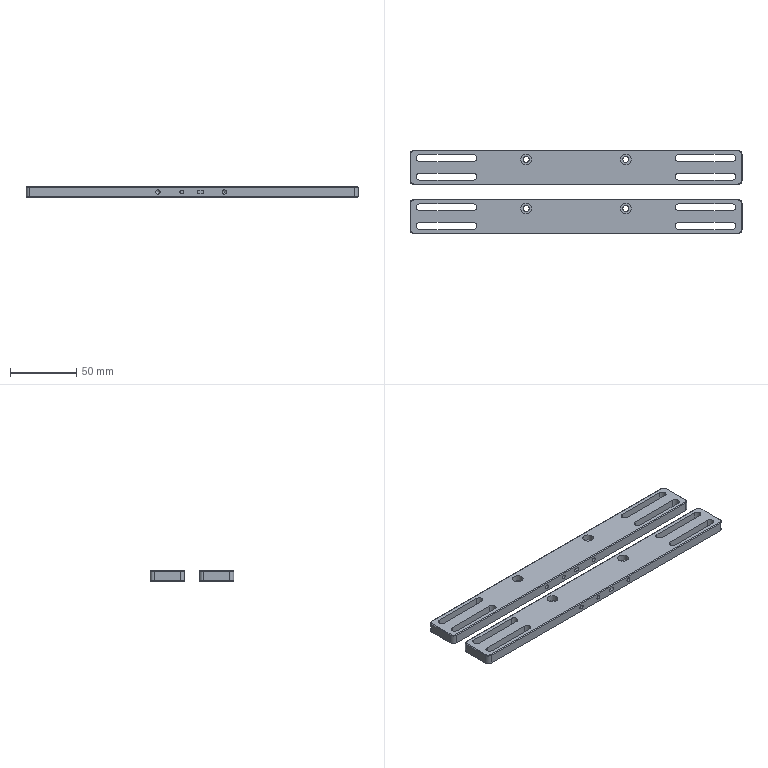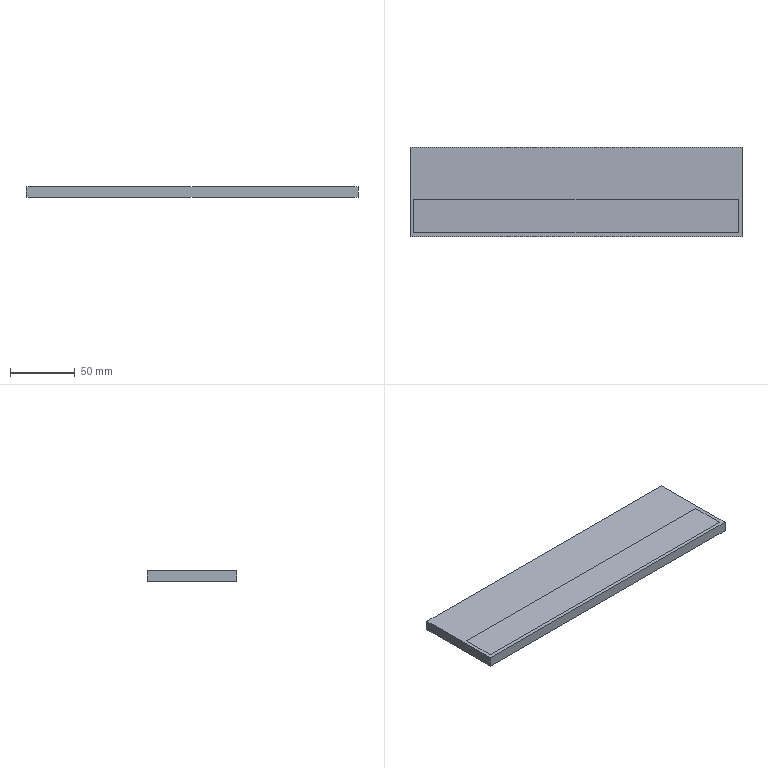CAM job | NX | 3+2 milling, drilling | part box 250 x 63 x 8 mm | stock box 256 x 69 x 8 mm
Tools:
number,name,description,diameter,corner_radius,flute_length,length,flutes
20,D10,Milling Tool-5 Parameters,10.0,0.0,50.0,75.0,2
22,D6A45,Milling Tool-5 Parameters,6.0,0.0,3.0,3.0,2
19,3.3ZT,Drilling Tool,3.2,0.0,35.0,50.0,2
24,4.5ZT,Drilling Tool,4.5,0.0,35.0,50.0,2
14,D4,Milling Tool-5 Parameters,4.0,0.0,50.0,75.0,2
17,D6,Milling Tool-5 Parameters,6.0,0.0,50.0,75.0,2
11,D10JING,Milling Tool-5 Parameters,10.0,0.0,50.0,75.0,2
12,D2,Milling Tool-5 Parameters,2.0,0.0,50.0,75.0,2
Operations:
program,operation,operation_type,tool,method,geometry_group,spindle_rpm,surface_speed,feed_per_tooth,feed_cut,feed_plunge,cut_length_mm,path_length_mm,cut_time_min,machine_time_min
1AB胶-255-70-8毛胚,ZLEVEL_PROFILE_COPY,ZLevelMilling,D10,METHOD,A,7500.0,235.0,0.1667,2500.0,100.0,9464.071,9786.657,3.786,3.818
1AB胶-255-70-8毛胚,DRILLING_COPY_1_COPY_1,Operation,D6A45,METHOD,A,5000.0,94.0,0.025,250.0,0.0,16.0,334.804,0.064,0.0959
1AB胶-255-70-8毛胚,DRILLING_COPY_1_COPY_COPY_COPY_COPY_1_COPY_COPY_1,Operation,4.5ZT,METHOD,A,2000.0,20.0,0.0375,150.0,0.0,55.408,329.118,0.3694,0.3968
1AB胶-255-70-8毛胚,HOLE_MILLING_COPY,CylinderMilling,D6,METHOD,A,7500.0,141.0,0.0933,1400.0,100.0,358.79,772.82,0.2563,0.2977
1AB胶-255-70-8毛胚,ZLEVEL_PROFILE_COPY_COPY_2,ZLevelMilling,D4,METHOD,A,7500.0,235.0,0.1667,2500.0,100.0,14040.272,14920.21,5.616,5.704
1AB胶-255-70-8毛胚,ZLEVEL_PROFILE_1_COPY_1_COPY_COPY,ZLevelMilling,D6A45,METHOD,A,7500.0,141.0,0.0667,1000.0,100.0,1986.386,4666.689,1.986,2.254
1AB胶-255-70-8毛胚,ZLEVEL_PROFILE_COPY_COPY_1,ZLevelMilling,D10JING,METHOD,A,7500.0,235.0,0.0667,1000.0,100.0,3550.292,3943.424,3.55,3.59
2,DRILLING_COPY_1_COPY_1_COPY,Operation,D6A45,METHOD,B,5000.0,94.0,0.025,250.0,0.0,16.0,151.822,0.064,0.0776
2,DRILLING_COPY_1_COPY_COPY_COPY_COPY_1_COPY,Operation,3.3ZT,METHOD,B,2000.0,20.0,0.0375,150.0,0.0,37.948,188.986,0.253,0.2681
2,ZLEVEL_PROFILE_COPY_COPY,ZLevelMilling,D2,METHOD,B,7500.0,47.0,0.0667,1000.0,100.0,565.762,718.711,0.5658,0.5811
2,ZLEVEL_PROFILE_1_COPY_1_COPY_COPY_COPY,ZLevelMilling,D6A45,METHOD,B,7500.0,141.0,0.0667,1000.0,100.0,32.327,351.651,0.0323,0.0643
2,刀补12,ZLevelMilling,D2,METHOD,B,7500.0,47.0,0.0667,1000.0,100.0,76.38,230.157,0.0764,0.0918